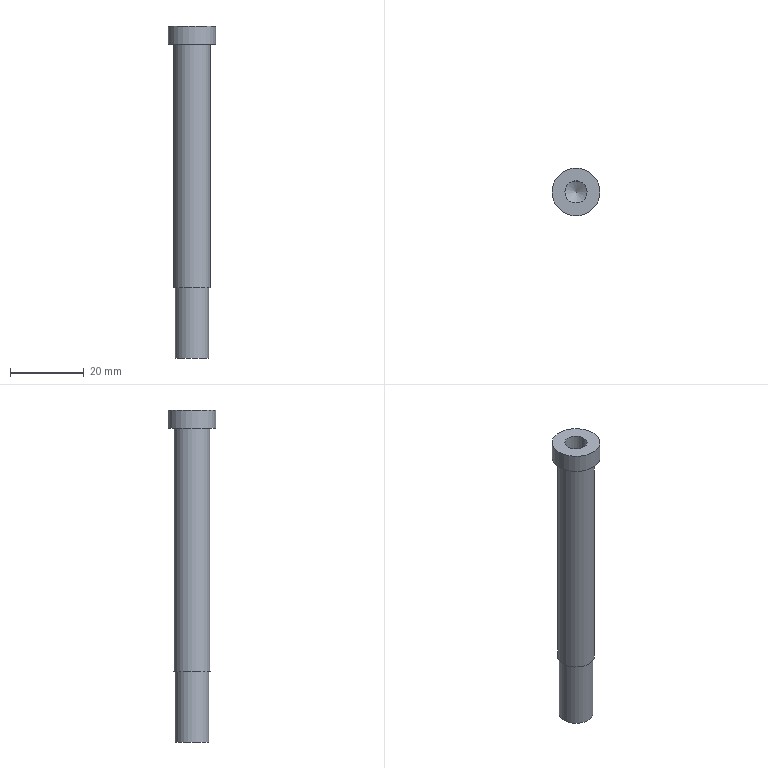Part | NX | features solid 2 | 1 solid | 9 faces | box 13 x 13 x 90 mm | volume 6699 mm3 | cylinder 4 | plane 4 | cone 1 | commonest cylinder face diameters 6 x1 9.1 x1 10 x1 13 x1
STEP:
#1=CARTESIAN_POINT('',(-284.143,-474.5,102.));
#2=VERTEX_POINT('',#1);
#3=CARTESIAN_POINT('',(-289.143,-474.5,102.));
#4=DIRECTION('',(0.,0.,1.));
#5=DIRECTION('',(1.,0.,0.));
#6=AXIS2_PLACEMENT_3D('',#3,#4,#5);
#7=CIRCLE('',#6,5.);
#8=EDGE_CURVE('',#2,#2,#7,.T.);
#9=ORIENTED_EDGE('',*,*,#8,.T.);
#10=EDGE_LOOP('',(#9));
#11=FACE_BOUND('',#10,.T.);
#12=CARTESIAN_POINT('',(-284.143,-474.5,168.));
#13=VERTEX_POINT('',#12);
#14=CARTESIAN_POINT('',(-289.143,-474.5,168.));
#15=DIRECTION('',(0.,0.,1.));
#16=DIRECTION('',(1.,0.,0.));
#17=AXIS2_PLACEMENT_3D('',#14,#15,#16);
#18=CIRCLE('',#17,5.);
#19=EDGE_CURVE('',#13,#13,#18,.T.);
#20=ORIENTED_EDGE('',*,*,#19,.F.);
#21=EDGE_LOOP('',(#20));
#22=FACE_BOUND('',#21,.T.);
#23=CARTESIAN_POINT('',(-289.143,-474.5,173.));
#24=DIRECTION('',(0.,0.,-1.));
#25=DIRECTION('',(-1.,0.,0.));
#26=AXIS2_PLACEMENT_3D('',#23,#24,#25);
#27=CYLINDRICAL_SURFACE('',#26,5.);
#28=ADVANCED_FACE('',(#11,#22),#27,.T.);
#29=CARTESIAN_POINT('',(-284.593,-474.5,102.));
#30=VERTEX_POINT('',#29);
#31=CARTESIAN_POINT('',(-289.143,-474.5,102.));
#32=DIRECTION('',(0.,0.,1.));
#33=DIRECTION('',(1.,0.,0.));
#34=AXIS2_PLACEMENT_3D('',#31,#32,#33);
#35=CIRCLE('',#34,4.55);
#36=EDGE_CURVE('',#30,#30,#35,.T.);
#37=ORIENTED_EDGE('',*,*,#36,.T.);
#38=EDGE_LOOP('',(#37));
#39=FACE_BOUND('',#38,.T.);
#40=ORIENTED_EDGE('',*,*,#8,.F.);
#41=EDGE_LOOP('',(#40));
#42=FACE_BOUND('',#41,.T.);
#43=CARTESIAN_POINT('',(-289.143,-474.5,102.));
#44=DIRECTION('',(0.,0.,1.));
#45=DIRECTION('',(1.,0.,0.));
#46=AXIS2_PLACEMENT_3D('',#43,#44,#45);
#47=PLANE('',#46);
#48=ADVANCED_FACE('',(#39,#42),#47,.F.);
#49=CARTESIAN_POINT('',(-282.643,-474.5,168.));
#50=VERTEX_POINT('',#49);
#51=CARTESIAN_POINT('',(-289.143,-474.5,168.));
#52=DIRECTION('',(0.,0.,1.));
#53=DIRECTION('',(1.,0.,0.));
#54=AXIS2_PLACEMENT_3D('',#51,#52,#53);
#55=CIRCLE('',#54,6.5);
#56=EDGE_CURVE('',#50,#50,#55,.T.);
#57=ORIENTED_EDGE('',*,*,#56,.F.);
#58=EDGE_LOOP('',(#57));
#59=FACE_BOUND('',#58,.T.);
#60=ORIENTED_EDGE('',*,*,#19,.T.);
#61=EDGE_LOOP('',(#60));
#62=FACE_BOUND('',#61,.T.);
#63=CARTESIAN_POINT('',(-289.143,-474.5,168.));
#64=DIRECTION('',(0.,0.,1.));
#65=DIRECTION('',(1.,0.,0.));
#66=AXIS2_PLACEMENT_3D('',#63,#64,#65);
#67=PLANE('',#66);
#68=ADVANCED_FACE('',(#59,#62),#67,.F.);
#69=ORIENTED_EDGE('',*,*,#56,.T.);
#70=EDGE_LOOP('',(#69));
#71=FACE_BOUND('',#70,.T.);
#72=CARTESIAN_POINT('',(-282.643,-474.5,173.));
#73=VERTEX_POINT('',#72);
#74=CARTESIAN_POINT('',(-289.143,-474.5,173.));
#75=DIRECTION('',(0.,0.,1.));
#76=DIRECTION('',(1.,0.,0.));
#77=AXIS2_PLACEMENT_3D('',#74,#75,#76);
#78=CIRCLE('',#77,6.5);
#79=EDGE_CURVE('',#73,#73,#78,.T.);
#80=ORIENTED_EDGE('',*,*,#79,.F.);
#81=EDGE_LOOP('',(#80));
#82=FACE_BOUND('',#81,.T.);
#83=CARTESIAN_POINT('',(-289.143,-474.5,168.));
#84=DIRECTION('',(0.,0.,1.));
#85=DIRECTION('',(1.,0.,0.));
#86=AXIS2_PLACEMENT_3D('',#83,#84,#85);
#87=CYLINDRICAL_SURFACE('',#86,6.5);
#88=ADVANCED_FACE('',(#71,#82),#87,.T.);
#89=CARTESIAN_POINT('',(-292.143,-474.5,173.));
#90=VERTEX_POINT('',#89);
#91=CARTESIAN_POINT('',(-289.143,-474.5,173.));
#92=DIRECTION('',(0.,0.,-1.));
#93=DIRECTION('',(-1.,0.,0.));
#94=AXIS2_PLACEMENT_3D('',#91,#92,#93);
#95=CIRCLE('',#94,3.);
#96=EDGE_CURVE('',#90,#90,#95,.T.);
#97=ORIENTED_EDGE('',*,*,#96,.T.);
#98=EDGE_LOOP('',(#97));
#99=FACE_BOUND('',#98,.T.);
#100=ORIENTED_EDGE('',*,*,#79,.T.);
#101=EDGE_LOOP('',(#100));
#102=FACE_BOUND('',#101,.T.);
#103=CARTESIAN_POINT('',(-289.143,-474.5,173.));
#104=DIRECTION('',(0.,0.,1.));
#105=DIRECTION('',(1.,0.,0.));
#106=AXIS2_PLACEMENT_3D('',#103,#104,#105);
#107=PLANE('',#106);
#108=ADVANCED_FACE('',(#99,#102),#107,.T.);
#109=CARTESIAN_POINT('',(-284.593,-474.5,83.));
#110=VERTEX_POINT('',#109);
#111=CARTESIAN_POINT('',(-289.143,-474.5,83.));
#112=DIRECTION('',(0.,0.,1.));
#113=DIRECTION('',(1.,0.,0.));
#114=AXIS2_PLACEMENT_3D('',#111,#112,#113);
#115=CIRCLE('',#114,4.55);
#116=EDGE_CURVE('',#110,#110,#115,.T.);
#117=ORIENTED_EDGE('',*,*,#116,.T.);
#118=EDGE_LOOP('',(#117));
#119=FACE_BOUND('',#118,.T.);
#120=ORIENTED_EDGE('',*,*,#36,.F.);
#121=EDGE_LOOP('',(#120));
#122=FACE_BOUND('',#121,.T.);
#123=CARTESIAN_POINT('',(-289.143,-474.5,83.));
#124=DIRECTION('',(0.,0.,1.));
#125=DIRECTION('',(1.,0.,0.));
#126=AXIS2_PLACEMENT_3D('',#123,#124,#125);
#127=CYLINDRICAL_SURFACE('',#126,4.55);
#128=ADVANCED_FACE('',(#119,#122),#127,.T.);
#129=ORIENTED_EDGE('',*,*,#116,.F.);
#130=EDGE_LOOP('',(#129));
#131=FACE_BOUND('',#130,.T.);
#132=CARTESIAN_POINT('',(-289.143,-474.5,83.));
#133=DIRECTION('',(0.,0.,1.));
#134=DIRECTION('',(1.,0.,0.));
#135=AXIS2_PLACEMENT_3D('',#132,#133,#134);
#136=PLANE('',#135);
#137=ADVANCED_FACE('',(#131),#136,.F.);
#138=CARTESIAN_POINT('',(-292.143,-474.5,160.));
#139=VERTEX_POINT('',#138);
#140=CARTESIAN_POINT('',(-289.143,-474.5,160.));
#141=DIRECTION('',(0.,0.,-1.));
#142=DIRECTION('',(-1.,0.,0.));
#143=AXIS2_PLACEMENT_3D('',#140,#141,#142);
#144=CIRCLE('',#143,3.);
#145=EDGE_CURVE('',#139,#139,#144,.T.);
#146=ORIENTED_EDGE('',*,*,#145,.F.);
#147=EDGE_LOOP('',(#146));
#148=FACE_BOUND('',#147,.T.);
#149=CARTESIAN_POINT('',(-289.143,-474.5,158.268));
#150=VERTEX_POINT('',#149);
#151=VERTEX_LOOP('',#150);
#152=FACE_BOUND('',#151,.T.);
#153=CARTESIAN_POINT('',(-289.143,-474.5,160.));
#154=DIRECTION('',(0.,0.,1.));
#155=DIRECTION('',(1.,0.,0.));
#156=AXIS2_PLACEMENT_3D('',#153,#154,#155);
#157=CONICAL_SURFACE('',#156,3.,1.047);
#158=ADVANCED_FACE('',(#148,#152),#157,.F.);
#159=ORIENTED_EDGE('',*,*,#145,.T.);
#160=EDGE_LOOP('',(#159));
#161=FACE_BOUND('',#160,.T.);
#162=ORIENTED_EDGE('',*,*,#96,.F.);
#163=EDGE_LOOP('',(#162));
#164=FACE_BOUND('',#163,.T.);
#165=CARTESIAN_POINT('',(-289.143,-474.5,173.));
#166=DIRECTION('',(0.,0.,-1.));
#167=DIRECTION('',(-1.,0.,0.));
#168=AXIS2_PLACEMENT_3D('',#165,#166,#167);
#169=CYLINDRICAL_SURFACE('',#168,3.);
#170=ADVANCED_FACE('',(#161,#164),#169,.F.);
#171=CLOSED_SHELL('',(#28,#48,#68,#88,#108,#128,#137,#158,#170));
#172=MANIFOLD_SOLID_BREP('',#171);
#173=(LENGTH_UNIT()NAMED_UNIT(*)SI_UNIT(.MILLI.,.METRE.));
#174=UNCERTAINTY_MEASURE_WITH_UNIT(LENGTH_MEASURE(0.00001),#173,'','');
#175=(NAMED_UNIT(*)PLANE_ANGLE_UNIT()SI_UNIT($,.RADIAN.));
#176=(NAMED_UNIT(*)SI_UNIT($,.STERADIAN.)SOLID_ANGLE_UNIT());
#177=(GEOMETRIC_REPRESENTATION_CONTEXT(3)GLOBAL_UNCERTAINTY_ASSIGNED_CONTEXT((#174))GLOBAL_UNIT_ASSIGNED_CONTEXT((#173,#175,#176))REPRESENTATION_CONTEXT('',''));
#178=ADVANCED_BREP_SHAPE_REPRESENTATION('',(#172),#177);